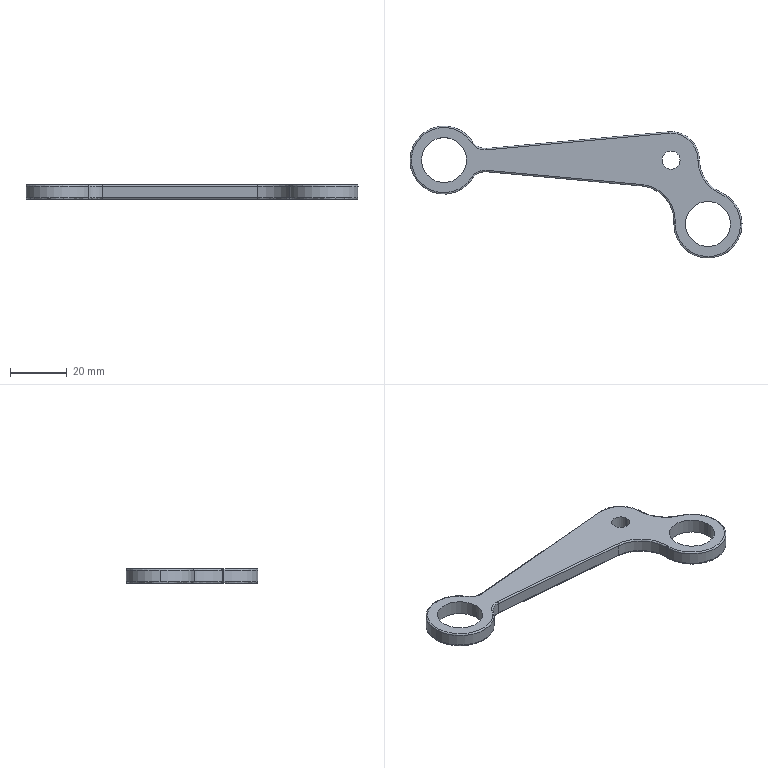Part | SolidWorks | features BaseBody 1 | 1 solid | 44 faces | box 117 x 46.517 x 5.08 mm | volume 8533 mm3 | cylinder 20 | spline 20 | plane 4 | commonest cylinder face diameters 24 x5 1.016 x4 15.875 x4 6.35 x2 10.16 x2 25 x2